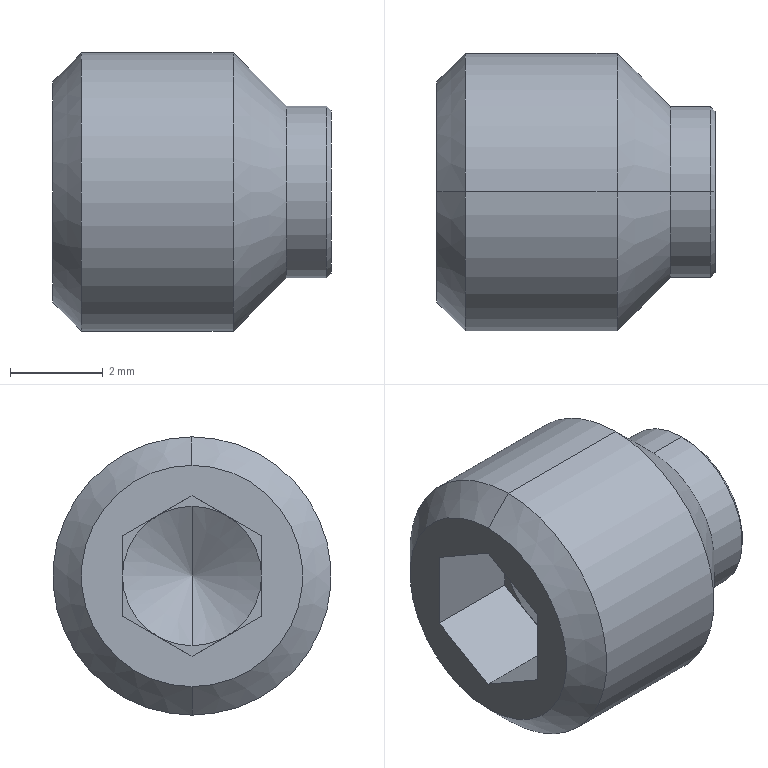Part | NX | features BREP 1 | 1 solid | 26 faces | box 6 x 6 x 6 mm | volume 120.9 mm3 | plane 14 | cone 8 | cylinder 4 | commonest cylinder face diameters 3.7 x2 6 x2